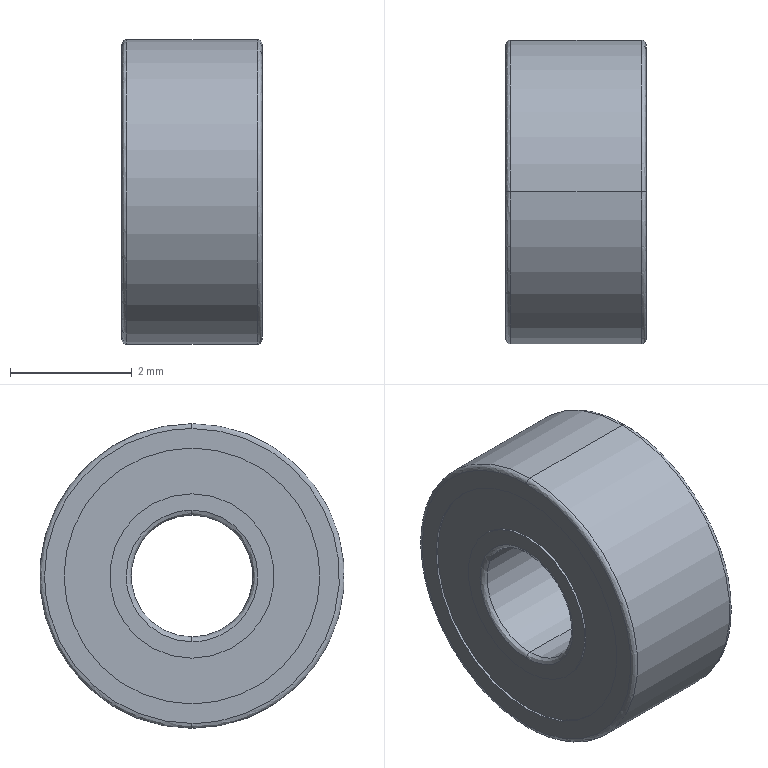Part | SolidWorks | features BaseBody 1 | 1 solid | 26 faces | box 2.3 x 5 x 5 mm | volume 37.258 mm3 | cylinder 12 | spline 8 | plane 6 | commonest cylinder face diameters 2.7 x4 4.2 x4 2 x2 5 x2
STEP:
#1=CARTESIAN_POINT('',(2.22,0.,-2.5));
#2=VERTEX_POINT('',#1);
#3=CARTESIAN_POINT('',(2.22,0.,2.5));
#4=VERTEX_POINT('',#3);
#5=CARTESIAN_POINT('',(2.22,0.,0.));
#6=DIRECTION('',(-1.,0.,0.));
#7=DIRECTION('',(0.,0.,-1.));
#8=AXIS2_PLACEMENT_3D('',#5,#6,#7);
#9=CIRCLE('',#8,2.5);
#10=EDGE_CURVE('',#2,#4,#9,.T.);
#11=ORIENTED_EDGE('',*,*,#10,.F.);
#12=CARTESIAN_POINT('',(2.3,0.,-2.42));
#13=VERTEX_POINT('',#12);
#14=CARTESIAN_POINT('',(2.22,0.,-2.42));
#15=DIRECTION('',(0.,-1.,0.));
#16=DIRECTION('',(0.,0.,-1.));
#17=AXIS2_PLACEMENT_3D('',#14,#15,#16);
#18=CIRCLE('',#17,0.08);
#19=EDGE_CURVE('',#2,#13,#18,.T.);
#20=ORIENTED_EDGE('',*,*,#19,.T.);
#21=CARTESIAN_POINT('',(2.3,0.,2.42));
#22=VERTEX_POINT('',#21);
#23=CARTESIAN_POINT('',(2.3,0.,-2.42));
#24=CARTESIAN_POINT('',(2.3,-4.84,-2.42));
#25=CARTESIAN_POINT('',(2.3,-4.84,2.42));
#26=CARTESIAN_POINT('',(2.3,0.,2.42));
#27=(BOUNDED_CURVE()B_SPLINE_CURVE(3,(#23,#24,#25,#26),.UNSPECIFIED.,.F.,.F.)B_SPLINE_CURVE_WITH_KNOTS((4,4),(0.,1.),.UNSPECIFIED.)CURVE()GEOMETRIC_REPRESENTATION_ITEM()RATIONAL_B_SPLINE_CURVE((1.,0.3333,0.3333,1.))REPRESENTATION_ITEM(''));
#28=EDGE_CURVE('',#13,#22,#27,.T.);
#29=ORIENTED_EDGE('',*,*,#28,.T.);
#30=CARTESIAN_POINT('',(2.22,0.,2.42));
#31=DIRECTION('',(0.,1.,0.));
#32=DIRECTION('',(0.,0.,1.));
#33=AXIS2_PLACEMENT_3D('',#30,#31,#32);
#34=CIRCLE('',#33,0.08);
#35=EDGE_CURVE('',#4,#22,#34,.T.);
#36=ORIENTED_EDGE('',*,*,#35,.F.);
#37=EDGE_LOOP('',(#11,#20,#29,#36));
#38=FACE_OUTER_BOUND('',#37,.T.);
#39=CARTESIAN_POINT('',(2.22,0.,-2.5));
#40=CARTESIAN_POINT('',(2.22,-5.,-2.5));
#41=CARTESIAN_POINT('',(2.22,-5.,2.5));
#42=CARTESIAN_POINT('',(2.22,0.,2.5));
#43=CARTESIAN_POINT('',(2.267,0.,-2.5));
#44=CARTESIAN_POINT('',(2.267,-5.,-2.5));
#45=CARTESIAN_POINT('',(2.267,-5.,2.5));
#46=CARTESIAN_POINT('',(2.267,0.,2.5));
#47=CARTESIAN_POINT('',(2.3,0.,-2.467));
#48=CARTESIAN_POINT('',(2.3,-4.934,-2.467));
#49=CARTESIAN_POINT('',(2.3,-4.934,2.467));
#50=CARTESIAN_POINT('',(2.3,0.,2.467));
#51=CARTESIAN_POINT('',(2.3,0.,-2.42));
#52=CARTESIAN_POINT('',(2.3,-4.84,-2.42));
#53=CARTESIAN_POINT('',(2.3,-4.84,2.42));
#54=CARTESIAN_POINT('',(2.3,0.,2.42));
#55=(BOUNDED_SURFACE()B_SPLINE_SURFACE(3,3,((#39,#40,#41,#42),(#43,#44,#45,#46),(#47,#48,#49,#50),(#51,#52,#53,#54)),.UNSPECIFIED.,.F.,.F.,.T.)B_SPLINE_SURFACE_WITH_KNOTS((4,4),(4,4),(0.,1.),(0.,1.),.UNSPECIFIED.)GEOMETRIC_REPRESENTATION_ITEM()RATIONAL_B_SPLINE_SURFACE(((1.,0.3333,0.3333,1.),(0.8047,0.2682,0.2682,0.8047),(0.8047,0.2682,0.2682,0.8047),(1.,0.3333,0.3333,1.)))REPRESENTATION_ITEM('')SURFACE());
#56=ADVANCED_FACE('',(#38),#55,.T.);
#57=CARTESIAN_POINT('',(0.,0.,2.42));
#58=VERTEX_POINT('',#57);
#59=CARTESIAN_POINT('',(0.,0.,-2.42));
#60=VERTEX_POINT('',#59);
#61=CARTESIAN_POINT('',(0.,0.,2.42));
#62=CARTESIAN_POINT('',(0.,-4.84,2.42));
#63=CARTESIAN_POINT('',(0.,-4.84,-2.42));
#64=CARTESIAN_POINT('',(0.,0.,-2.42));
#65=(BOUNDED_CURVE()B_SPLINE_CURVE(3,(#61,#62,#63,#64),.UNSPECIFIED.,.F.,.T.)B_SPLINE_CURVE_WITH_KNOTS((4,4),(0.,1.),.UNSPECIFIED.)CURVE()GEOMETRIC_REPRESENTATION_ITEM()RATIONAL_B_SPLINE_CURVE((1.,0.3333,0.3333,1.))REPRESENTATION_ITEM(''));
#66=EDGE_CURVE('',#58,#60,#65,.T.);
#67=ORIENTED_EDGE('',*,*,#66,.T.);
#68=CARTESIAN_POINT('',(0.08,0.,-2.5));
#69=VERTEX_POINT('',#68);
#70=CARTESIAN_POINT('',(0.08,0.,-2.42));
#71=DIRECTION('',(0.,-1.,0.));
#72=DIRECTION('',(0.,0.,-1.));
#73=AXIS2_PLACEMENT_3D('',#70,#71,#72);
#74=CIRCLE('',#73,0.08);
#75=EDGE_CURVE('',#60,#69,#74,.T.);
#76=ORIENTED_EDGE('',*,*,#75,.T.);
#77=CARTESIAN_POINT('',(0.08,0.,2.5));
#78=VERTEX_POINT('',#77);
#79=CARTESIAN_POINT('',(0.08,0.,0.));
#80=DIRECTION('',(1.,0.,0.));
#81=DIRECTION('',(0.,0.,-1.));
#82=AXIS2_PLACEMENT_3D('',#79,#80,#81);
#83=CIRCLE('',#82,2.5);
#84=EDGE_CURVE('',#78,#69,#83,.T.);
#85=ORIENTED_EDGE('',*,*,#84,.F.);
#86=CARTESIAN_POINT('',(0.08,0.,2.42));
#87=DIRECTION('',(0.,1.,0.));
#88=DIRECTION('',(0.,0.,1.));
#89=AXIS2_PLACEMENT_3D('',#86,#87,#88);
#90=CIRCLE('',#89,0.08);
#91=EDGE_CURVE('',#58,#78,#90,.T.);
#92=ORIENTED_EDGE('',*,*,#91,.F.);
#93=EDGE_LOOP('',(#67,#76,#85,#92));
#94=FACE_OUTER_BOUND('',#93,.T.);
#95=CARTESIAN_POINT('',(0.,0.,-2.42));
#96=CARTESIAN_POINT('',(0.,-4.84,-2.42));
#97=CARTESIAN_POINT('',(0.,-4.84,2.42));
#98=CARTESIAN_POINT('',(0.,0.,2.42));
#99=CARTESIAN_POINT('',(0.,0.,-2.467));
#100=CARTESIAN_POINT('',(0.,-4.934,-2.467));
#101=CARTESIAN_POINT('',(0.,-4.934,2.467));
#102=CARTESIAN_POINT('',(0.,0.,2.467));
#103=CARTESIAN_POINT('',(0.03314,0.,-2.5));
#104=CARTESIAN_POINT('',(0.03314,-5.,-2.5));
#105=CARTESIAN_POINT('',(0.03314,-5.,2.5));
#106=CARTESIAN_POINT('',(0.03314,0.,2.5));
#107=CARTESIAN_POINT('',(0.08,0.,-2.5));
#108=CARTESIAN_POINT('',(0.08,-5.,-2.5));
#109=CARTESIAN_POINT('',(0.08,-5.,2.5));
#110=CARTESIAN_POINT('',(0.08,0.,2.5));
#111=(BOUNDED_SURFACE()B_SPLINE_SURFACE(3,3,((#95,#96,#97,#98),(#99,#100,#101,#102),(#103,#104,#105,#106),(#107,#108,#109,#110)),.UNSPECIFIED.,.F.,.F.,.F.)B_SPLINE_SURFACE_WITH_KNOTS((4,4),(4,4),(0.,1.),(0.,1.),.UNSPECIFIED.)GEOMETRIC_REPRESENTATION_ITEM()RATIONAL_B_SPLINE_SURFACE(((1.,0.3333,0.3333,1.),(0.8047,0.2682,0.2682,0.8047),(0.8047,0.2682,0.2682,0.8047),(1.,0.3333,0.3333,1.)))REPRESENTATION_ITEM('')SURFACE());
#112=ADVANCED_FACE('',(#94),#111,.T.);
#113=CARTESIAN_POINT('',(2.3,0.,-1.08));
#114=VERTEX_POINT('',#113);
#115=CARTESIAN_POINT('',(2.3,0.,1.08));
#116=VERTEX_POINT('',#115);
#117=CARTESIAN_POINT('',(2.3,0.,-1.08));
#118=CARTESIAN_POINT('',(2.3,-0.06875,-1.08));
#119=CARTESIAN_POINT('',(2.3,-0.17,-1.07));
#120=CARTESIAN_POINT('',(2.3,-0.2849,-1.043));
#121=CARTESIAN_POINT('',(2.3,-0.3334,-1.027));
#122=CARTESIAN_POINT('',(2.3,-0.3656,-1.016));
#123=CARTESIAN_POINT('',(2.3,-0.3802,-1.011));
#124=CARTESIAN_POINT('',(2.3,-0.5359,-0.9495));
#125=CARTESIAN_POINT('',(2.3,-0.6584,-0.8688));
#126=CARTESIAN_POINT('',(2.3,-0.8163,-0.7111));
#127=CARTESIAN_POINT('',(2.3,-0.8858,-0.6259));
#128=CARTESIAN_POINT('',(2.3,-0.9505,-0.5154));
#129=CARTESIAN_POINT('',(2.3,-0.9747,-0.4657));
#130=CARTESIAN_POINT('',(2.3,-0.99,-0.432));
#131=CARTESIAN_POINT('',(2.3,-0.9979,-0.4135));
#132=CARTESIAN_POINT('',(2.3,-1.055,-0.2702));
#133=CARTESIAN_POINT('',(2.3,-1.08,-0.137));
#134=CARTESIAN_POINT('',(2.3,-1.08,0.06849));
#135=CARTESIAN_POINT('',(2.3,-1.071,0.1696));
#136=CARTESIAN_POINT('',(2.3,-1.043,0.2845));
#137=CARTESIAN_POINT('',(2.3,-1.028,0.3332));
#138=CARTESIAN_POINT('',(2.3,-1.016,0.3655));
#139=CARTESIAN_POINT('',(2.3,-1.011,0.3802));
#140=CARTESIAN_POINT('',(2.3,-0.9495,0.5359));
#141=CARTESIAN_POINT('',(2.3,-0.8688,0.6584));
#142=CARTESIAN_POINT('',(2.3,-0.7111,0.8163));
#143=CARTESIAN_POINT('',(2.3,-0.6259,0.8858));
#144=CARTESIAN_POINT('',(2.3,-0.5154,0.9505));
#145=CARTESIAN_POINT('',(2.3,-0.4657,0.9747));
#146=CARTESIAN_POINT('',(2.3,-0.432,0.99));
#147=CARTESIAN_POINT('',(2.3,-0.4134,0.9979));
#148=CARTESIAN_POINT('',(2.3,-0.2704,1.055));
#149=CARTESIAN_POINT('',(2.3,-0.1379,1.08));
#150=CARTESIAN_POINT('',(2.3,0.,1.08));
#151=B_SPLINE_CURVE_WITH_KNOTS('',3,(#117,#118,#119,#120,#121,#122,#123,#124,#125,#126,#127,#128,#129,#130,#131,#132,#133,#134,#135,#136,#137,#138,#139,#140,#141,#142,#143,#144,#145,#146,#147,#148,#149,#150),.UNSPECIFIED.,.F.,.F.,(4,1,1,2,2,2,1,1,2,2,2,1,1,2,2,2,1,1,2,2,4),(0.,0.0625,0.09375,0.1094,0.125,0.25,0.3125,0.3438,0.3594,0.375,0.5,0.5625,0.5938,0.6094,0.625,0.75,0.8125,0.8438,0.8594,0.875,1.),.UNSPECIFIED.);
#152=EDGE_CURVE('',#114,#116,#151,.T.);
#153=ORIENTED_EDGE('',*,*,#152,.F.);
#154=CARTESIAN_POINT('',(2.22,0.,-1.));
#155=VERTEX_POINT('',#154);
#156=CARTESIAN_POINT('',(2.22,0.,-1.08));
#157=DIRECTION('',(0.,-1.,0.));
#158=DIRECTION('',(0.,0.,-1.));
#159=AXIS2_PLACEMENT_3D('',#156,#157,#158);
#160=CIRCLE('',#159,0.08);
#161=EDGE_CURVE('',#114,#155,#160,.T.);
#162=ORIENTED_EDGE('',*,*,#161,.T.);
#163=CARTESIAN_POINT('',(2.22,0.,1.));
#164=VERTEX_POINT('',#163);
#165=CARTESIAN_POINT('',(2.22,0.,0.));
#166=DIRECTION('',(-1.,0.,0.));
#167=DIRECTION('',(0.,0.,1.));
#168=AXIS2_PLACEMENT_3D('',#165,#166,#167);
#169=CIRCLE('',#168,1.);
#170=EDGE_CURVE('',#155,#164,#169,.T.);
#171=ORIENTED_EDGE('',*,*,#170,.T.);
#172=CARTESIAN_POINT('',(2.22,0.,1.08));
#173=DIRECTION('',(0.,1.,0.));
#174=DIRECTION('',(0.,0.,1.));
#175=AXIS2_PLACEMENT_3D('',#172,#173,#174);
#176=CIRCLE('',#175,0.08);
#177=EDGE_CURVE('',#116,#164,#176,.T.);
#178=ORIENTED_EDGE('',*,*,#177,.F.);
#179=EDGE_LOOP('',(#153,#162,#171,#178));
#180=FACE_OUTER_BOUND('',#179,.T.);
#181=CARTESIAN_POINT('',(2.3,0.,-1.08));
#182=CARTESIAN_POINT('',(2.3,-2.16,-1.08));
#183=CARTESIAN_POINT('',(2.3,-2.16,1.08));
#184=CARTESIAN_POINT('',(2.3,0.,1.08));
#185=CARTESIAN_POINT('',(2.3,0.,-1.033));
#186=CARTESIAN_POINT('',(2.3,-2.066,-1.033));
#187=CARTESIAN_POINT('',(2.3,-2.066,1.033));
#188=CARTESIAN_POINT('',(2.3,0.,1.033));
#189=CARTESIAN_POINT('',(2.267,0.,-1.));
#190=CARTESIAN_POINT('',(2.267,-2.,-1.));
#191=CARTESIAN_POINT('',(2.267,-2.,1.));
#192=CARTESIAN_POINT('',(2.267,0.,1.));
#193=CARTESIAN_POINT('',(2.22,0.,-1.));
#194=CARTESIAN_POINT('',(2.22,-2.,-1.));
#195=CARTESIAN_POINT('',(2.22,-2.,1.));
#196=CARTESIAN_POINT('',(2.22,0.,1.));
#197=(BOUNDED_SURFACE()B_SPLINE_SURFACE(3,3,((#181,#182,#183,#184),(#185,#186,#187,#188),(#189,#190,#191,#192),(#193,#194,#195,#196)),.UNSPECIFIED.,.F.,.F.,.T.)B_SPLINE_SURFACE_WITH_KNOTS((4,4),(4,4),(0.,1.),(0.,1.),.UNSPECIFIED.)GEOMETRIC_REPRESENTATION_ITEM()RATIONAL_B_SPLINE_SURFACE(((1.,0.3333,0.3333,1.),(0.8047,0.2682,0.2682,0.8047),(0.8047,0.2682,0.2682,0.8047),(1.,0.3333,0.3333,1.)))REPRESENTATION_ITEM('')SURFACE());
#198=ADVANCED_FACE('',(#180),#197,.T.);
#199=CARTESIAN_POINT('',(0.08,0.,1.));
#200=VERTEX_POINT('',#199);
#201=CARTESIAN_POINT('',(0.08,0.,-1.));
#202=VERTEX_POINT('',#201);
#203=CARTESIAN_POINT('',(0.08,0.,0.));
#204=DIRECTION('',(1.,0.,0.));
#205=DIRECTION('',(0.,0.,1.));
#206=AXIS2_PLACEMENT_3D('',#203,#204,#205);
#207=CIRCLE('',#206,1.);
#208=EDGE_CURVE('',#200,#202,#207,.T.);
#209=ORIENTED_EDGE('',*,*,#208,.T.);
#210=CARTESIAN_POINT('',(0.,0.,-1.08));
#211=VERTEX_POINT('',#210);
#212=CARTESIAN_POINT('',(0.08,0.,-1.08));
#213=DIRECTION('',(0.,-1.,0.));
#214=DIRECTION('',(0.,0.,-1.));
#215=AXIS2_PLACEMENT_3D('',#212,#213,#214);
#216=CIRCLE('',#215,0.08);
#217=EDGE_CURVE('',#202,#211,#216,.T.);
#218=ORIENTED_EDGE('',*,*,#217,.T.);
#219=CARTESIAN_POINT('',(0.,0.,1.08));
#220=VERTEX_POINT('',#219);
#221=CARTESIAN_POINT('',(0.,0.,1.08));
#222=CARTESIAN_POINT('',(0.,-0.06875,1.08));
#223=CARTESIAN_POINT('',(0.,-0.17,1.07));
#224=CARTESIAN_POINT('',(0.,-0.2849,1.043));
#225=CARTESIAN_POINT('',(0.,-0.3334,1.027));
#226=CARTESIAN_POINT('',(0.,-0.3656,1.016));
#227=CARTESIAN_POINT('',(0.,-0.3802,1.011));
#228=CARTESIAN_POINT('',(0.,-0.5359,0.9495));
#229=CARTESIAN_POINT('',(0.,-0.6584,0.8688));
#230=CARTESIAN_POINT('',(0.,-0.8163,0.7111));
#231=CARTESIAN_POINT('',(0.,-0.8858,0.6259));
#232=CARTESIAN_POINT('',(0.,-0.9505,0.5154));
#233=CARTESIAN_POINT('',(0.,-0.9747,0.4657));
#234=CARTESIAN_POINT('',(0.,-0.99,0.432));
#235=CARTESIAN_POINT('',(0.,-0.9979,0.4135));
#236=CARTESIAN_POINT('',(0.,-1.055,0.2702));
#237=CARTESIAN_POINT('',(0.,-1.08,0.137));
#238=CARTESIAN_POINT('',(0.,-1.08,-0.06849));
#239=CARTESIAN_POINT('',(0.,-1.071,-0.1696));
#240=CARTESIAN_POINT('',(0.,-1.043,-0.2845));
#241=CARTESIAN_POINT('',(0.,-1.028,-0.3332));
#242=CARTESIAN_POINT('',(0.,-1.016,-0.3655));
#243=CARTESIAN_POINT('',(0.,-1.011,-0.3802));
#244=CARTESIAN_POINT('',(0.,-0.9495,-0.5359));
#245=CARTESIAN_POINT('',(0.,-0.8688,-0.6584));
#246=CARTESIAN_POINT('',(0.,-0.7111,-0.8163));
#247=CARTESIAN_POINT('',(0.,-0.6259,-0.8858));
#248=CARTESIAN_POINT('',(0.,-0.5154,-0.9505));
#249=CARTESIAN_POINT('',(0.,-0.4657,-0.9747));
#250=CARTESIAN_POINT('',(0.,-0.432,-0.99));
#251=CARTESIAN_POINT('',(0.,-0.4134,-0.9979));
#252=CARTESIAN_POINT('',(0.,-0.2704,-1.055));
#253=CARTESIAN_POINT('',(0.,-0.1379,-1.08));
#254=CARTESIAN_POINT('',(0.,0.,-1.08));
#255=B_SPLINE_CURVE_WITH_KNOTS('',3,(#221,#222,#223,#224,#225,#226,#227,#228,#229,#230,#231,#232,#233,#234,#235,#236,#237,#238,#239,#240,#241,#242,#243,#244,#245,#246,#247,#248,#249,#250,#251,#252,#253,#254),.UNSPECIFIED.,.F.,.F.,(4,1,1,2,2,2,1,1,2,2,2,1,1,2,2,2,1,1,2,2,4),(0.,0.0625,0.09375,0.1094,0.125,0.25,0.3125,0.3438,0.3594,0.375,0.5,0.5625,0.5938,0.6094,0.625,0.75,0.8125,0.8438,0.8594,0.875,1.),.UNSPECIFIED.);
#256=EDGE_CURVE('',#220,#211,#255,.T.);
#257=ORIENTED_EDGE('',*,*,#256,.F.);
#258=CARTESIAN_POINT('',(0.08,0.,1.08));
#259=DIRECTION('',(0.,1.,0.));
#260=DIRECTION('',(0.,0.,1.));
#261=AXIS2_PLACEMENT_3D('',#258,#259,#260);
#262=CIRCLE('',#261,0.08);
#263=EDGE_CURVE('',#200,#220,#262,.T.);
#264=ORIENTED_EDGE('',*,*,#263,.F.);
#265=EDGE_LOOP('',(#209,#218,#257,#264));
#266=FACE_OUTER_BOUND('',#265,.T.);
#267=CARTESIAN_POINT('',(0.08,0.,-1.));
#268=CARTESIAN_POINT('',(0.08,-2.,-1.));
#269=CARTESIAN_POINT('',(0.08,-2.,1.));
#270=CARTESIAN_POINT('',(0.08,0.,1.));
#271=CARTESIAN_POINT('',(0.03314,0.,-1.));
#272=CARTESIAN_POINT('',(0.03314,-2.,-1.));
#273=CARTESIAN_POINT('',(0.03314,-2.,1.));
#274=CARTESIAN_POINT('',(0.03314,0.,1.));
#275=CARTESIAN_POINT('',(0.,0.,-1.033));
#276=CARTESIAN_POINT('',(0.,-2.066,-1.033));
#277=CARTESIAN_POINT('',(0.,-2.066,1.033));
#278=CARTESIAN_POINT('',(0.,0.,1.033));
#279=CARTESIAN_POINT('',(0.,0.,-1.08));
#280=CARTESIAN_POINT('',(0.,-2.16,-1.08));
#281=CARTESIAN_POINT('',(0.,-2.16,1.08));
#282=CARTESIAN_POINT('',(0.,0.,1.08));
#283=(BOUNDED_SURFACE()B_SPLINE_SURFACE(3,3,((#267,#268,#269,#270),(#271,#272,#273,#274),(#275,#276,#277,#278),(#279,#280,#281,#282)),.UNSPECIFIED.,.F.,.F.,.F.)B_SPLINE_SURFACE_WITH_KNOTS((4,4),(4,4),(0.,1.),(0.,1.),.UNSPECIFIED.)GEOMETRIC_REPRESENTATION_ITEM()RATIONAL_B_SPLINE_SURFACE(((1.,0.3333,0.3333,1.),(0.8047,0.2682,0.2682,0.8047),(0.8047,0.2682,0.2682,0.8047),(1.,0.3333,0.3333,1.)))REPRESENTATION_ITEM('')SURFACE());
#284=ADVANCED_FACE('',(#266),#283,.T.);
#285=CARTESIAN_POINT('',(0.08,0.,0.));
#286=DIRECTION('',(1.,0.,0.));
#287=DIRECTION('',(0.,0.,-1.));
#288=AXIS2_PLACEMENT_3D('',#285,#286,#287);
#289=CIRCLE('',#288,2.5);
#290=EDGE_CURVE('',#69,#78,#289,.T.);
#291=ORIENTED_EDGE('',*,*,#290,.T.);
#292=CARTESIAN_POINT('',(1.15,0.,2.5));
#293=DIRECTION('',(1.,0.,0.));
#294=VECTOR('',#293,1000.);
#295=LINE('',#292,#294);
#296=EDGE_CURVE('',#78,#4,#295,.T.);
#297=ORIENTED_EDGE('',*,*,#296,.T.);
#298=CARTESIAN_POINT('',(2.22,0.,0.));
#299=DIRECTION('',(-1.,0.,0.));
#300=DIRECTION('',(0.,0.,-1.));
#301=AXIS2_PLACEMENT_3D('',#298,#299,#300);
#302=CIRCLE('',#301,2.5);
#303=EDGE_CURVE('',#4,#2,#302,.T.);
#304=ORIENTED_EDGE('',*,*,#303,.T.);
#305=CARTESIAN_POINT('',(1.15,0.,-2.5));
#306=DIRECTION('',(1.,0.,0.));
#307=VECTOR('',#306,1000.);
#308=LINE('',#305,#307);
#309=EDGE_CURVE('',#69,#2,#308,.T.);
#310=ORIENTED_EDGE('',*,*,#309,.F.);
#311=EDGE_LOOP('',(#291,#297,#304,#310));
#312=FACE_OUTER_BOUND('',#311,.T.);
#313=CARTESIAN_POINT('',(1.15,0.,0.));
#314=DIRECTION('',(1.,0.,0.));
#315=DIRECTION('',(0.,0.,-1.));
#316=AXIS2_PLACEMENT_3D('',#313,#314,#315);
#317=CYLINDRICAL_SURFACE('',#316,2.5);
#318=ADVANCED_FACE('',(#312),#317,.T.);
#319=CARTESIAN_POINT('',(2.262,0.,2.1));
#320=VERTEX_POINT('',#319);
#321=CARTESIAN_POINT('',(2.262,0.,-2.1));
#322=VERTEX_POINT('',#321);
#323=CARTESIAN_POINT('',(2.262,0.,0.));
#324=DIRECTION('',(1.,0.,0.));
#325=DIRECTION('',(0.,0.,-1.));
#326=AXIS2_PLACEMENT_3D('',#323,#324,#325);
#327=CIRCLE('',#326,2.1);
#328=EDGE_CURVE('',#320,#322,#327,.T.);
#329=ORIENTED_EDGE('',*,*,#328,.F.);
#330=CARTESIAN_POINT('',(2.3,0.,2.1));
#331=VERTEX_POINT('',#330);
#332=CARTESIAN_POINT('',(2.281,0.,2.1));
#333=DIRECTION('',(1.,0.,0.));
#334=VECTOR('',#333,1000.);
#335=LINE('',#332,#334);
#336=EDGE_CURVE('',#320,#331,#335,.T.);
#337=ORIENTED_EDGE('',*,*,#336,.T.);
#338=CARTESIAN_POINT('',(2.3,0.,-2.1));
#339=VERTEX_POINT('',#338);
#340=CARTESIAN_POINT('',(2.3,0.,0.));
#341=DIRECTION('',(-1.,0.,0.));
#342=DIRECTION('',(0.,0.,-1.));
#343=AXIS2_PLACEMENT_3D('',#340,#341,#342);
#344=CIRCLE('',#343,2.1);
#345=EDGE_CURVE('',#339,#331,#344,.T.);
#346=ORIENTED_EDGE('',*,*,#345,.F.);
#347=CARTESIAN_POINT('',(2.281,0.,-2.1));
#348=DIRECTION('',(1.,0.,0.));
#349=VECTOR('',#348,1000.);
#350=LINE('',#347,#349);
#351=EDGE_CURVE('',#322,#339,#350,.T.);
#352=ORIENTED_EDGE('',*,*,#351,.F.);
#353=EDGE_LOOP('',(#329,#337,#346,#352));
#354=FACE_OUTER_BOUND('',#353,.T.);
#355=CARTESIAN_POINT('',(2.281,0.,0.));
#356=DIRECTION('',(1.,0.,0.));
#357=DIRECTION('',(0.,0.,-1.));
#358=AXIS2_PLACEMENT_3D('',#355,#356,#357);
#359=CYLINDRICAL_SURFACE('',#358,2.1);
#360=ADVANCED_FACE('',(#354),#359,.F.);
#361=CARTESIAN_POINT('',(0.,0.,2.1));
#362=VERTEX_POINT('',#361);
#363=CARTESIAN_POINT('',(0.,0.,-2.1));
#364=VERTEX_POINT('',#363);
#365=CARTESIAN_POINT('',(0.,0.,0.));
#366=DIRECTION('',(1.,0.,0.));
#367=DIRECTION('',(0.,0.,-1.));
#368=AXIS2_PLACEMENT_3D('',#365,#366,#367);
#369=CIRCLE('',#368,2.1);
#370=EDGE_CURVE('',#362,#364,#369,.T.);
#371=ORIENTED_EDGE('',*,*,#370,.F.);
#372=CARTESIAN_POINT('',(0.0382,0.,2.1));
#373=VERTEX_POINT('',#372);
#374=CARTESIAN_POINT('',(0.0191,0.,2.1));
#375=DIRECTION('',(1.,0.,0.));
#376=VECTOR('',#375,1000.);
#377=LINE('',#374,#376);
#378=EDGE_CURVE('',#362,#373,#377,.T.);
#379=ORIENTED_EDGE('',*,*,#378,.T.);
#380=CARTESIAN_POINT('',(0.0382,0.,-2.1));
#381=VERTEX_POINT('',#380);
#382=CARTESIAN_POINT('',(0.0382,0.,0.));
#383=DIRECTION('',(-1.,0.,0.));
#384=DIRECTION('',(0.,0.,-1.));
#385=AXIS2_PLACEMENT_3D('',#382,#383,#384);
#386=CIRCLE('',#385,2.1);
#387=EDGE_CURVE('',#381,#373,#386,.T.);
#388=ORIENTED_EDGE('',*,*,#387,.F.);
#389=CARTESIAN_POINT('',(0.0191,0.,-2.1));
#390=DIRECTION('',(1.,0.,0.));
#391=VECTOR('',#390,1000.);
#392=LINE('',#389,#391);
#393=EDGE_CURVE('',#364,#381,#392,.T.);
#394=ORIENTED_EDGE('',*,*,#393,.F.);
#395=EDGE_LOOP('',(#371,#379,#388,#394));
#396=FACE_OUTER_BOUND('',#395,.T.);
#397=CARTESIAN_POINT('',(0.0191,0.,0.));
#398=DIRECTION('',(1.,0.,0.));
#399=DIRECTION('',(0.,0.,-1.));
#400=AXIS2_PLACEMENT_3D('',#397,#398,#399);
#401=CYLINDRICAL_SURFACE('',#400,2.1);
#402=ADVANCED_FACE('',(#396),#401,.F.);
#403=CARTESIAN_POINT('',(2.262,0.,1.35));
#404=VERTEX_POINT('',#403);
#405=CARTESIAN_POINT('',(2.262,0.,-1.35));
#406=VERTEX_POINT('',#405);
#407=CARTESIAN_POINT('',(2.262,0.,0.));
#408=DIRECTION('',(-1.,0.,0.));
#409=DIRECTION('',(0.,0.,-1.));
#410=AXIS2_PLACEMENT_3D('',#407,#408,#409);
#411=CIRCLE('',#410,1.35);
#412=EDGE_CURVE('',#404,#406,#411,.T.);
#413=ORIENTED_EDGE('',*,*,#412,.F.);
#414=CARTESIAN_POINT('',(2.3,0.,1.35));
#415=VERTEX_POINT('',#414);
#416=CARTESIAN_POINT('',(2.281,0.,1.35));
#417=DIRECTION('',(1.,0.,0.));
#418=VECTOR('',#417,1000.);
#419=LINE('',#416,#418);
#420=EDGE_CURVE('',#404,#415,#419,.T.);
#421=ORIENTED_EDGE('',*,*,#420,.T.);
#422=CARTESIAN_POINT('',(2.3,0.,-1.35));
#423=VERTEX_POINT('',#422);
#424=CARTESIAN_POINT('',(2.3,0.,0.));
#425=DIRECTION('',(-1.,0.,0.));
#426=DIRECTION('',(0.,0.,-1.));
#427=AXIS2_PLACEMENT_3D('',#424,#425,#426);
#428=CIRCLE('',#427,1.35);
#429=EDGE_CURVE('',#415,#423,#428,.T.);
#430=ORIENTED_EDGE('',*,*,#429,.T.);
#431=CARTESIAN_POINT('',(2.281,0.,-1.35));
#432=DIRECTION('',(1.,0.,0.));
#433=VECTOR('',#432,1000.);
#434=LINE('',#431,#433);
#435=EDGE_CURVE('',#406,#423,#434,.T.);
#436=ORIENTED_EDGE('',*,*,#435,.F.);
#437=EDGE_LOOP('',(#413,#421,#430,#436));
#438=FACE_OUTER_BOUND('',#437,.T.);
#439=CARTESIAN_POINT('',(2.281,0.,0.));
#440=DIRECTION('',(1.,0.,0.));
#441=DIRECTION('',(0.,0.,-1.));
#442=AXIS2_PLACEMENT_3D('',#439,#440,#441);
#443=CYLINDRICAL_SURFACE('',#442,1.35);
#444=ADVANCED_FACE('',(#438),#443,.T.);
#445=CARTESIAN_POINT('',(0.,0.,-1.35));
#446=VERTEX_POINT('',#445);
#447=CARTESIAN_POINT('',(0.,0.,1.35));
#448=VERTEX_POINT('',#447);
#449=CARTESIAN_POINT('',(0.,0.,0.));
#450=DIRECTION('',(1.,0.,0.));
#451=DIRECTION('',(0.,0.,-1.));
#452=AXIS2_PLACEMENT_3D('',#449,#450,#451);
#453=CIRCLE('',#452,1.35);
#454=EDGE_CURVE('',#446,#448,#453,.T.);
#455=ORIENTED_EDGE('',*,*,#454,.T.);
#456=CARTESIAN_POINT('',(0.0382,0.,1.35));
#457=VERTEX_POINT('',#456);
#458=CARTESIAN_POINT('',(0.0191,0.,1.35));
#459=DIRECTION('',(1.,0.,0.));
#460=VECTOR('',#459,1000.);
#461=LINE('',#458,#460);
#462=EDGE_CURVE('',#448,#457,#461,.T.);
#463=ORIENTED_EDGE('',*,*,#462,.T.);
#464=CARTESIAN_POINT('',(0.0382,0.,-1.35));
#465=VERTEX_POINT('',#464);
#466=CARTESIAN_POINT('',(0.0382,0.,0.));
#467=DIRECTION('',(1.,0.,0.));
#468=DIRECTION('',(0.,0.,-1.));
#469=AXIS2_PLACEMENT_3D('',#466,#467,#468);
#470=CIRCLE('',#469,1.35);
#471=EDGE_CURVE('',#465,#457,#470,.T.);
#472=ORIENTED_EDGE('',*,*,#471,.F.);
#473=CARTESIAN_POINT('',(0.0191,0.,-1.35));
#474=DIRECTION('',(1.,0.,0.));
#475=VECTOR('',#474,1000.);
#476=LINE('',#473,#475);
#477=EDGE_CURVE('',#446,#465,#476,.T.);
#478=ORIENTED_EDGE('',*,*,#477,.F.);
#479=EDGE_LOOP('',(#455,#463,#472,#478));
#480=FACE_OUTER_BOUND('',#479,.T.);
#481=CARTESIAN_POINT('',(0.0191,0.,0.));
#482=DIRECTION('',(1.,0.,0.));
#483=DIRECTION('',(0.,0.,-1.));
#484=AXIS2_PLACEMENT_3D('',#481,#482,#483);
#485=CYLINDRICAL_SURFACE('',#484,1.35);
#486=ADVANCED_FACE('',(#480),#485,.T.);
#487=ORIENTED_EDGE('',*,*,#208,.F.);
#488=CARTESIAN_POINT('',(1.15,0.,1.));
#489=DIRECTION('',(1.,0.,0.));
#490=VECTOR('',#489,1000.);
#491=LINE('',#488,#490);
#492=EDGE_CURVE('',#200,#164,#491,.T.);
#493=ORIENTED_EDGE('',*,*,#492,.T.);
#494=ORIENTED_EDGE('',*,*,#170,.F.);
#495=CARTESIAN_POINT('',(1.15,0.,-1.));
#496=DIRECTION('',(1.,0.,0.));
#497=VECTOR('',#496,1000.);
#498=LINE('',#495,#497);
#499=EDGE_CURVE('',#202,#155,#498,.T.);
#500=ORIENTED_EDGE('',*,*,#499,.F.);
#501=EDGE_LOOP('',(#487,#493,#494,#500));
#502=FACE_OUTER_BOUND('',#501,.T.);
#503=CARTESIAN_POINT('',(1.15,0.,0.));
#504=DIRECTION('',(1.,0.,0.));
#505=DIRECTION('',(0.,0.,-1.));
#506=AXIS2_PLACEMENT_3D('',#503,#504,#505);
#507=CYLINDRICAL_SURFACE('',#506,1.);
#508=ADVANCED_FACE('',(#502),#507,.F.);
#509=ORIENTED_EDGE('',*,*,#296,.F.);
#510=ORIENTED_EDGE('',*,*,#84,.T.);
#511=ORIENTED_EDGE('',*,*,#309,.T.);
#512=ORIENTED_EDGE('',*,*,#10,.T.);
#513=EDGE_LOOP('',(#509,#510,#511,#512));
#514=FACE_OUTER_BOUND('',#513,.T.);
#515=CARTESIAN_POINT('',(1.15,0.,0.));
#516=DIRECTION('',(1.,0.,0.));
#517=DIRECTION('',(0.,0.,-1.));
#518=AXIS2_PLACEMENT_3D('',#515,#516,#517);
#519=CYLINDRICAL_SURFACE('',#518,2.5);
#520=ADVANCED_FACE('',(#514),#519,.T.);
#521=ORIENTED_EDGE('',*,*,#19,.F.);
#522=ORIENTED_EDGE('',*,*,#303,.F.);
#523=ORIENTED_EDGE('',*,*,#35,.T.);
#524=CARTESIAN_POINT('',(2.3,2.42,0.));
#525=VERTEX_POINT('',#524);
#526=CARTESIAN_POINT('',(2.3,0.,2.42));
#527=CARTESIAN_POINT('',(2.3,1.418,2.42));
#528=CARTESIAN_POINT('',(2.3,2.42,1.418));
#529=CARTESIAN_POINT('',(2.3,2.42,0.));
#530=(BOUNDED_CURVE()B_SPLINE_CURVE(3,(#526,#527,#528,#529),.UNSPECIFIED.,.F.,.T.)B_SPLINE_CURVE_WITH_KNOTS((4,4),(0.,1.),.UNSPECIFIED.)CURVE()GEOMETRIC_REPRESENTATION_ITEM()RATIONAL_B_SPLINE_CURVE((1.,0.8047,0.8047,1.))REPRESENTATION_ITEM(''));
#531=EDGE_CURVE('',#22,#525,#530,.T.);
#532=ORIENTED_EDGE('',*,*,#531,.T.);
#533=CARTESIAN_POINT('',(2.3,2.42,0.));
#534=CARTESIAN_POINT('',(2.3,2.42,-1.418));
#535=CARTESIAN_POINT('',(2.3,1.418,-2.42));
#536=CARTESIAN_POINT('',(2.3,0.,-2.42));
#537=(BOUNDED_CURVE()B_SPLINE_CURVE(3,(#533,#534,#535,#536),.UNSPECIFIED.,.F.,.F.)B_SPLINE_CURVE_WITH_KNOTS((4,4),(0.,1.),.UNSPECIFIED.)CURVE()GEOMETRIC_REPRESENTATION_ITEM()RATIONAL_B_SPLINE_CURVE((1.,0.8047,0.8047,1.))REPRESENTATION_ITEM(''));
#538=EDGE_CURVE('',#525,#13,#537,.T.);
#539=ORIENTED_EDGE('',*,*,#538,.T.);
#540=EDGE_LOOP('',(#521,#522,#523,#532,#539));
#541=FACE_OUTER_BOUND('',#540,.T.);
#542=CARTESIAN_POINT('',(2.22,0.,2.5));
#543=CARTESIAN_POINT('',(2.22,5.,2.5));
#544=CARTESIAN_POINT('',(2.22,5.,-2.5));
#545=CARTESIAN_POINT('',(2.22,0.,-2.5));
#546=CARTESIAN_POINT('',(2.267,0.,2.5));
#547=CARTESIAN_POINT('',(2.267,5.,2.5));
#548=CARTESIAN_POINT('',(2.267,5.,-2.5));
#549=CARTESIAN_POINT('',(2.267,0.,-2.5));
#550=CARTESIAN_POINT('',(2.3,0.,2.467));
#551=CARTESIAN_POINT('',(2.3,4.934,2.467));
#552=CARTESIAN_POINT('',(2.3,4.934,-2.467));
#553=CARTESIAN_POINT('',(2.3,0.,-2.467));
#554=CARTESIAN_POINT('',(2.3,0.,2.42));
#555=CARTESIAN_POINT('',(2.3,4.84,2.42));
#556=CARTESIAN_POINT('',(2.3,4.84,-2.42));
#557=CARTESIAN_POINT('',(2.3,0.,-2.42));
#558=(BOUNDED_SURFACE()B_SPLINE_SURFACE(3,3,((#542,#543,#544,#545),(#546,#547,#548,#549),(#550,#551,#552,#553),(#554,#555,#556,#557)),.UNSPECIFIED.,.F.,.F.,.T.)B_SPLINE_SURFACE_WITH_KNOTS((4,4),(4,4),(0.,1.),(0.,1.),.UNSPECIFIED.)GEOMETRIC_REPRESENTATION_ITEM()RATIONAL_B_SPLINE_SURFACE(((1.,0.3333,0.3333,1.),(0.8047,0.2682,0.2682,0.8047),(0.8047,0.2682,0.2682,0.8047),(1.,0.3333,0.3333,1.)))REPRESENTATION_ITEM('')SURFACE());
#559=ADVANCED_FACE('',(#541),#558,.T.);
#560=ORIENTED_EDGE('',*,*,#75,.F.);
#561=CARTESIAN_POINT('',(0.,2.42,0.));
#562=VERTEX_POINT('',#561);
#563=CARTESIAN_POINT('',(0.,0.,-2.42));
#564=CARTESIAN_POINT('',(0.,1.418,-2.42));
#565=CARTESIAN_POINT('',(0.,2.42,-1.418));
#566=CARTESIAN_POINT('',(0.,2.42,0.));
#567=(BOUNDED_CURVE()B_SPLINE_CURVE(3,(#563,#564,#565,#566),.UNSPECIFIED.,.F.,.T.)B_SPLINE_CURVE_WITH_KNOTS((4,4),(0.,1.),.UNSPECIFIED.)CURVE()GEOMETRIC_REPRESENTATION_ITEM()RATIONAL_B_SPLINE_CURVE((1.,0.8047,0.8047,1.))REPRESENTATION_ITEM(''));
#568=EDGE_CURVE('',#60,#562,#567,.T.);
#569=ORIENTED_EDGE('',*,*,#568,.T.);
#570=CARTESIAN_POINT('',(0.,2.42,0.));
#571=CARTESIAN_POINT('',(0.,2.42,1.418));
#572=CARTESIAN_POINT('',(0.,1.418,2.42));
#573=CARTESIAN_POINT('',(0.,0.,2.42));
#574=(BOUNDED_CURVE()B_SPLINE_CURVE(3,(#570,#571,#572,#573),.UNSPECIFIED.,.F.,.T.)B_SPLINE_CURVE_WITH_KNOTS((4,4),(0.,1.),.UNSPECIFIED.)CURVE()GEOMETRIC_REPRESENTATION_ITEM()RATIONAL_B_SPLINE_CURVE((1.,0.8047,0.8047,1.))REPRESENTATION_ITEM(''));
#575=EDGE_CURVE('',#562,#58,#574,.T.);
#576=ORIENTED_EDGE('',*,*,#575,.T.);
#577=ORIENTED_EDGE('',*,*,#91,.T.);
#578=ORIENTED_EDGE('',*,*,#290,.F.);
#579=EDGE_LOOP('',(#560,#569,#576,#577,#578));
#580=FACE_OUTER_BOUND('',#579,.T.);
#581=CARTESIAN_POINT('',(0.,0.,2.42));
#582=CARTESIAN_POINT('',(0.,4.84,2.42));
#583=CARTESIAN_POINT('',(0.,4.84,-2.42));
#584=CARTESIAN_POINT('',(0.,0.,-2.42));
#585=CARTESIAN_POINT('',(0.,0.,2.467));
#586=CARTESIAN_POINT('',(0.,4.934,2.467));
#587=CARTESIAN_POINT('',(0.,4.934,-2.467));
#588=CARTESIAN_POINT('',(0.,0.,-2.467));
#589=CARTESIAN_POINT('',(0.03314,0.,2.5));
#590=CARTESIAN_POINT('',(0.03314,5.,2.5));
#591=CARTESIAN_POINT('',(0.03314,5.,-2.5));
#592=CARTESIAN_POINT('',(0.03314,0.,-2.5));
#593=CARTESIAN_POINT('',(0.08,0.,2.5));
#594=CARTESIAN_POINT('',(0.08,5.,2.5));
#595=CARTESIAN_POINT('',(0.08,5.,-2.5));
#596=CARTESIAN_POINT('',(0.08,0.,-2.5));
#597=(BOUNDED_SURFACE()B_SPLINE_SURFACE(3,3,((#581,#582,#583,#584),(#585,#586,#587,#588),(#589,#590,#591,#592),(#593,#594,#595,#596)),.UNSPECIFIED.,.F.,.F.,.T.)B_SPLINE_SURFACE_WITH_KNOTS((4,4),(4,4),(0.,1.),(0.,1.),.UNSPECIFIED.)GEOMETRIC_REPRESENTATION_ITEM()RATIONAL_B_SPLINE_SURFACE(((1.,0.3333,0.3333,1.),(0.8047,0.2682,0.2682,0.8047),(0.8047,0.2682,0.2682,0.8047),(1.,0.3333,0.3333,1.)))REPRESENTATION_ITEM('')SURFACE());
#598=ADVANCED_FACE('',(#580),#597,.T.);
#599=ORIENTED_EDGE('',*,*,#345,.T.);
#600=CARTESIAN_POINT('',(2.3,0.,0.));
#601=DIRECTION('',(-1.,0.,0.));
#602=DIRECTION('',(0.,0.,-1.));
#603=AXIS2_PLACEMENT_3D('',#600,#601,#602);
#604=CIRCLE('',#603,2.1);
#605=EDGE_CURVE('',#331,#339,#604,.T.);
#606=ORIENTED_EDGE('',*,*,#605,.T.);
#607=EDGE_LOOP('',(#599,#606));
#608=FACE_BOUND('',#607,.T.);
#609=ORIENTED_EDGE('',*,*,#531,.F.);
#610=ORIENTED_EDGE('',*,*,#28,.F.);
#611=ORIENTED_EDGE('',*,*,#538,.F.);
#612=EDGE_LOOP('',(#609,#610,#611));
#613=FACE_OUTER_BOUND('',#612,.T.);
#614=CARTESIAN_POINT('',(2.3,2.26,0.));
#615=DIRECTION('',(1.,0.,0.));
#616=DIRECTION('',(0.,0.,-1.));
#617=AXIS2_PLACEMENT_3D('',#614,#615,#616);
#618=PLANE('',#617);
#619=ADVANCED_FACE('',(#608,#613),#618,.T.);
#620=ORIENTED_EDGE('',*,*,#66,.F.);
#621=ORIENTED_EDGE('',*,*,#575,.F.);
#622=ORIENTED_EDGE('',*,*,#568,.F.);
#623=EDGE_LOOP('',(#620,#621,#622));
#624=FACE_OUTER_BOUND('',#623,.T.);
#625=CARTESIAN_POINT('',(0.,0.,0.));
#626=DIRECTION('',(1.,0.,0.));
#627=DIRECTION('',(0.,0.,-1.));
#628=AXIS2_PLACEMENT_3D('',#625,#626,#627);
#629=CIRCLE('',#628,2.1);
#630=EDGE_CURVE('',#364,#362,#629,.T.);
#631=ORIENTED_EDGE('',*,*,#630,.T.);
#632=ORIENTED_EDGE('',*,*,#370,.T.);
#633=EDGE_LOOP('',(#631,#632));
#634=FACE_BOUND('',#633,.T.);
#635=CARTESIAN_POINT('',(0.,2.26,0.));
#636=DIRECTION('',(-1.,0.,0.));
#637=DIRECTION('',(0.,0.,1.));
#638=AXIS2_PLACEMENT_3D('',#635,#636,#637);
#639=PLANE('',#638);
#640=ADVANCED_FACE('',(#624,#634),#639,.T.);
#641=ORIENTED_EDGE('',*,*,#336,.F.);
#642=CARTESIAN_POINT('',(2.262,0.,0.));
#643=DIRECTION('',(1.,0.,0.));
#644=DIRECTION('',(0.,0.,-1.));
#645=AXIS2_PLACEMENT_3D('',#642,#643,#644);
#646=CIRCLE('',#645,2.1);
#647=EDGE_CURVE('',#322,#320,#646,.T.);
#648=ORIENTED_EDGE('',*,*,#647,.F.);
#649=ORIENTED_EDGE('',*,*,#351,.T.);
#650=ORIENTED_EDGE('',*,*,#605,.F.);
#651=EDGE_LOOP('',(#641,#648,#649,#650));
#652=FACE_OUTER_BOUND('',#651,.T.);
#653=CARTESIAN_POINT('',(2.281,0.,0.));
#654=DIRECTION('',(1.,0.,0.));
#655=DIRECTION('',(0.,0.,-1.));
#656=AXIS2_PLACEMENT_3D('',#653,#654,#655);
#657=CYLINDRICAL_SURFACE('',#656,2.1);
#658=ADVANCED_FACE('',(#652),#657,.F.);
#659=ORIENTED_EDGE('',*,*,#378,.F.);
#660=ORIENTED_EDGE('',*,*,#630,.F.);
#661=ORIENTED_EDGE('',*,*,#393,.T.);
#662=CARTESIAN_POINT('',(0.0382,0.,0.));
#663=DIRECTION('',(-1.,0.,0.));
#664=DIRECTION('',(0.,0.,-1.));
#665=AXIS2_PLACEMENT_3D('',#662,#663,#664);
#666=CIRCLE('',#665,2.1);
#667=EDGE_CURVE('',#373,#381,#666,.T.);
#668=ORIENTED_EDGE('',*,*,#667,.F.);
#669=EDGE_LOOP('',(#659,#660,#661,#668));
#670=FACE_OUTER_BOUND('',#669,.T.);
#671=CARTESIAN_POINT('',(0.0191,0.,0.));
#672=DIRECTION('',(1.,0.,0.));
#673=DIRECTION('',(0.,0.,-1.));
#674=AXIS2_PLACEMENT_3D('',#671,#672,#673);
#675=CYLINDRICAL_SURFACE('',#674,2.1);
#676=ADVANCED_FACE('',(#670),#675,.F.);
#677=CARTESIAN_POINT('',(2.262,0.,0.));
#678=DIRECTION('',(-1.,0.,0.));
#679=DIRECTION('',(0.,0.,-1.));
#680=AXIS2_PLACEMENT_3D('',#677,#678,#679);
#681=CIRCLE('',#680,1.35);
#682=EDGE_CURVE('',#406,#404,#681,.T.);
#683=ORIENTED_EDGE('',*,*,#682,.T.);
#684=ORIENTED_EDGE('',*,*,#412,.T.);
#685=EDGE_LOOP('',(#683,#684));
#686=FACE_BOUND('',#685,.T.);
#687=ORIENTED_EDGE('',*,*,#647,.T.);
#688=ORIENTED_EDGE('',*,*,#328,.T.);
#689=EDGE_LOOP('',(#687,#688));
#690=FACE_OUTER_BOUND('',#689,.T.);
#691=CARTESIAN_POINT('',(2.262,1.725,0.));
#692=DIRECTION('',(1.,0.,0.));
#693=DIRECTION('',(0.,0.,-1.));
#694=AXIS2_PLACEMENT_3D('',#691,#692,#693);
#695=PLANE('',#694);
#696=ADVANCED_FACE('',(#686,#690),#695,.T.);
#697=ORIENTED_EDGE('',*,*,#387,.T.);
#698=ORIENTED_EDGE('',*,*,#667,.T.);
#699=EDGE_LOOP('',(#697,#698));
#700=FACE_OUTER_BOUND('',#699,.T.);
#701=ORIENTED_EDGE('',*,*,#471,.T.);
#702=CARTESIAN_POINT('',(0.0382,0.,0.));
#703=DIRECTION('',(1.,0.,0.));
#704=DIRECTION('',(0.,0.,-1.));
#705=AXIS2_PLACEMENT_3D('',#702,#703,#704);
#706=CIRCLE('',#705,1.35);
#707=EDGE_CURVE('',#457,#465,#706,.T.);
#708=ORIENTED_EDGE('',*,*,#707,.T.);
#709=EDGE_LOOP('',(#701,#708));
#710=FACE_BOUND('',#709,.T.);
#711=CARTESIAN_POINT('',(0.0382,1.725,0.));
#712=DIRECTION('',(-1.,0.,0.));
#713=DIRECTION('',(0.,0.,1.));
#714=AXIS2_PLACEMENT_3D('',#711,#712,#713);
#715=PLANE('',#714);
#716=ADVANCED_FACE('',(#700,#710),#715,.T.);
#717=ORIENTED_EDGE('',*,*,#420,.F.);
#718=ORIENTED_EDGE('',*,*,#682,.F.);
#719=ORIENTED_EDGE('',*,*,#435,.T.);
#720=CARTESIAN_POINT('',(2.3,0.,0.));
#721=DIRECTION('',(-1.,0.,0.));
#722=DIRECTION('',(0.,0.,-1.));
#723=AXIS2_PLACEMENT_3D('',#720,#721,#722);
#724=CIRCLE('',#723,1.35);
#725=EDGE_CURVE('',#423,#415,#724,.T.);
#726=ORIENTED_EDGE('',*,*,#725,.T.);
#727=EDGE_LOOP('',(#717,#718,#719,#726));
#728=FACE_OUTER_BOUND('',#727,.T.);
#729=CARTESIAN_POINT('',(2.281,0.,0.));
#730=DIRECTION('',(1.,0.,0.));
#731=DIRECTION('',(0.,0.,-1.));
#732=AXIS2_PLACEMENT_3D('',#729,#730,#731);
#733=CYLINDRICAL_SURFACE('',#732,1.35);
#734=ADVANCED_FACE('',(#728),#733,.T.);
#735=ORIENTED_EDGE('',*,*,#462,.F.);
#736=CARTESIAN_POINT('',(0.,0.,0.));
#737=DIRECTION('',(1.,0.,0.));
#738=DIRECTION('',(0.,0.,-1.));
#739=AXIS2_PLACEMENT_3D('',#736,#737,#738);
#740=CIRCLE('',#739,1.35);
#741=EDGE_CURVE('',#448,#446,#740,.T.);
#742=ORIENTED_EDGE('',*,*,#741,.T.);
#743=ORIENTED_EDGE('',*,*,#477,.T.);
#744=ORIENTED_EDGE('',*,*,#707,.F.);
#745=EDGE_LOOP('',(#735,#742,#743,#744));
#746=FACE_OUTER_BOUND('',#745,.T.);
#747=CARTESIAN_POINT('',(0.0191,0.,0.));
#748=DIRECTION('',(1.,0.,0.));
#749=DIRECTION('',(0.,0.,-1.));
#750=AXIS2_PLACEMENT_3D('',#747,#748,#749);
#751=CYLINDRICAL_SURFACE('',#750,1.35);
#752=ADVANCED_FACE('',(#746),#751,.T.);
#753=ORIENTED_EDGE('',*,*,#152,.T.);
#754=CARTESIAN_POINT('',(2.3,1.08,0.));
#755=VERTEX_POINT('',#754);
#756=CARTESIAN_POINT('',(2.3,0.,1.08));
#757=CARTESIAN_POINT('',(2.3,0.06875,1.08));
#758=CARTESIAN_POINT('',(2.3,0.17,1.07));
#759=CARTESIAN_POINT('',(2.3,0.2849,1.043));
#760=CARTESIAN_POINT('',(2.3,0.3334,1.027));
#761=CARTESIAN_POINT('',(2.3,0.3656,1.016));
#762=CARTESIAN_POINT('',(2.3,0.3802,1.011));
#763=CARTESIAN_POINT('',(2.3,0.5359,0.9495));
#764=CARTESIAN_POINT('',(2.3,0.6584,0.8688));
#765=CARTESIAN_POINT('',(2.3,0.8163,0.7111));
#766=CARTESIAN_POINT('',(2.3,0.8858,0.6259));
#767=CARTESIAN_POINT('',(2.3,0.9505,0.5154));
#768=CARTESIAN_POINT('',(2.3,0.9747,0.4657));
#769=CARTESIAN_POINT('',(2.3,0.99,0.432));
#770=CARTESIAN_POINT('',(2.3,0.9979,0.4134));
#771=CARTESIAN_POINT('',(2.3,1.055,0.2704));
#772=CARTESIAN_POINT('',(2.3,1.08,0.1379));
#773=CARTESIAN_POINT('',(2.3,1.08,0.));
#774=B_SPLINE_CURVE_WITH_KNOTS('',3,(#756,#757,#758,#759,#760,#761,#762,#763,#764,#765,#766,#767,#768,#769,#770,#771,#772,#773),.UNSPECIFIED.,.F.,.F.,(4,1,1,2,2,2,1,1,2,2,4),(0.,0.125,0.1875,0.2188,0.25,0.5,0.625,0.6875,0.7187,0.75,1.),.UNSPECIFIED.);
#775=EDGE_CURVE('',#116,#755,#774,.T.);
#776=ORIENTED_EDGE('',*,*,#775,.T.);
#777=CARTESIAN_POINT('',(2.3,1.08,0.));
#778=CARTESIAN_POINT('',(2.3,1.08,-0.06875));
#779=CARTESIAN_POINT('',(2.3,1.07,-0.17));
#780=CARTESIAN_POINT('',(2.3,1.043,-0.2849));
#781=CARTESIAN_POINT('',(2.3,1.027,-0.3334));
#782=CARTESIAN_POINT('',(2.3,1.016,-0.3656));
#783=CARTESIAN_POINT('',(2.3,1.011,-0.3802));
#784=CARTESIAN_POINT('',(2.3,0.9495,-0.5359));
#785=CARTESIAN_POINT('',(2.3,0.8688,-0.6584));
#786=CARTESIAN_POINT('',(2.3,0.7111,-0.8163));
#787=CARTESIAN_POINT('',(2.3,0.6259,-0.8858));
#788=CARTESIAN_POINT('',(2.3,0.5154,-0.9505));
#789=CARTESIAN_POINT('',(2.3,0.4657,-0.9747));
#790=CARTESIAN_POINT('',(2.3,0.432,-0.99));
#791=CARTESIAN_POINT('',(2.3,0.4134,-0.9979));
#792=CARTESIAN_POINT('',(2.3,0.2704,-1.055));
#793=CARTESIAN_POINT('',(2.3,0.1379,-1.08));
#794=CARTESIAN_POINT('',(2.3,0.,-1.08));
#795=B_SPLINE_CURVE_WITH_KNOTS('',3,(#777,#778,#779,#780,#781,#782,#783,#784,#785,#786,#787,#788,#789,#790,#791,#792,#793,#794),.UNSPECIFIED.,.F.,.F.,(4,1,1,2,2,2,1,1,2,2,4),(0.,0.125,0.1875,0.2187,0.25,0.5,0.625,0.6875,0.7188,0.75,1.),.UNSPECIFIED.);
#796=EDGE_CURVE('',#755,#114,#795,.T.);
#797=ORIENTED_EDGE('',*,*,#796,.T.);
#798=EDGE_LOOP('',(#753,#776,#797));
#799=FACE_BOUND('',#798,.T.);
#800=ORIENTED_EDGE('',*,*,#725,.F.);
#801=ORIENTED_EDGE('',*,*,#429,.F.);
#802=EDGE_LOOP('',(#800,#801));
#803=FACE_OUTER_BOUND('',#802,.T.);
#804=CARTESIAN_POINT('',(2.3,1.215,0.));
#805=DIRECTION('',(1.,0.,0.));
#806=DIRECTION('',(0.,0.,-1.));
#807=AXIS2_PLACEMENT_3D('',#804,#805,#806);
#808=PLANE('',#807);
#809=ADVANCED_FACE('',(#799,#803),#808,.T.);
#810=ORIENTED_EDGE('',*,*,#454,.F.);
#811=ORIENTED_EDGE('',*,*,#741,.F.);
#812=EDGE_LOOP('',(#810,#811));
#813=FACE_OUTER_BOUND('',#812,.T.);
#814=CARTESIAN_POINT('',(0.,1.08,0.));
#815=VERTEX_POINT('',#814);
#816=CARTESIAN_POINT('',(0.,1.08,0.));
#817=CARTESIAN_POINT('',(0.,1.08,0.06875));
#818=CARTESIAN_POINT('',(0.,1.07,0.17));
#819=CARTESIAN_POINT('',(0.,1.043,0.2849));
#820=CARTESIAN_POINT('',(0.,1.027,0.3334));
#821=CARTESIAN_POINT('',(0.,1.016,0.3656));
#822=CARTESIAN_POINT('',(0.,1.011,0.3802));
#823=CARTESIAN_POINT('',(0.,0.9495,0.5359));
#824=CARTESIAN_POINT('',(0.,0.8688,0.6584));
#825=CARTESIAN_POINT('',(0.,0.7111,0.8163));
#826=CARTESIAN_POINT('',(0.,0.6259,0.8858));
#827=CARTESIAN_POINT('',(0.,0.5154,0.9505));
#828=CARTESIAN_POINT('',(0.,0.4657,0.9747));
#829=CARTESIAN_POINT('',(0.,0.432,0.99));
#830=CARTESIAN_POINT('',(0.,0.4134,0.9979));
#831=CARTESIAN_POINT('',(0.,0.2704,1.055));
#832=CARTESIAN_POINT('',(0.,0.1379,1.08));
#833=CARTESIAN_POINT('',(0.,0.,1.08));
#834=B_SPLINE_CURVE_WITH_KNOTS('',3,(#816,#817,#818,#819,#820,#821,#822,#823,#824,#825,#826,#827,#828,#829,#830,#831,#832,#833),.UNSPECIFIED.,.F.,.F.,(4,1,1,2,2,2,1,1,2,2,4),(0.,0.125,0.1875,0.2188,0.25,0.5,0.625,0.6875,0.7188,0.75,1.),.UNSPECIFIED.);
#835=EDGE_CURVE('',#815,#220,#834,.T.);
#836=ORIENTED_EDGE('',*,*,#835,.T.);
#837=ORIENTED_EDGE('',*,*,#256,.T.);
#838=CARTESIAN_POINT('',(0.,0.,-1.08));
#839=CARTESIAN_POINT('',(0.,0.06875,-1.08));
#840=CARTESIAN_POINT('',(0.,0.17,-1.07));
#841=CARTESIAN_POINT('',(0.,0.2849,-1.043));
#842=CARTESIAN_POINT('',(0.,0.3334,-1.027));
#843=CARTESIAN_POINT('',(0.,0.3656,-1.016));
#844=CARTESIAN_POINT('',(0.,0.3802,-1.011));
#845=CARTESIAN_POINT('',(0.,0.5359,-0.9495));
#846=CARTESIAN_POINT('',(0.,0.6584,-0.8688));
#847=CARTESIAN_POINT('',(0.,0.8163,-0.7111));
#848=CARTESIAN_POINT('',(0.,0.8858,-0.6259));
#849=CARTESIAN_POINT('',(0.,0.9505,-0.5154));
#850=CARTESIAN_POINT('',(0.,0.9747,-0.4657));
#851=CARTESIAN_POINT('',(0.,0.99,-0.432));
#852=CARTESIAN_POINT('',(0.,0.9979,-0.4134));
#853=CARTESIAN_POINT('',(0.,1.055,-0.2704));
#854=CARTESIAN_POINT('',(0.,1.08,-0.1379));
#855=CARTESIAN_POINT('',(0.,1.08,0.));
#856=B_SPLINE_CURVE_WITH_KNOTS('',3,(#838,#839,#840,#841,#842,#843,#844,#845,#846,#847,#848,#849,#850,#851,#852,#853,#854,#855),.UNSPECIFIED.,.F.,.F.,(4,1,1,2,2,2,1,1,2,2,4),(0.,0.125,0.1875,0.2188,0.25,0.5,0.625,0.6875,0.7187,0.75,1.),.UNSPECIFIED.);
#857=EDGE_CURVE('',#211,#815,#856,.T.);
#858=ORIENTED_EDGE('',*,*,#857,.T.);
#859=EDGE_LOOP('',(#836,#837,#858));
#860=FACE_BOUND('',#859,.T.);
#861=CARTESIAN_POINT('',(0.,1.215,0.));
#862=DIRECTION('',(-1.,0.,0.));
#863=DIRECTION('',(0.,0.,1.));
#864=AXIS2_PLACEMENT_3D('',#861,#862,#863);
#865=PLANE('',#864);
#866=ADVANCED_FACE('',(#813,#860),#865,.T.);
#867=ORIENTED_EDGE('',*,*,#161,.F.);
#868=ORIENTED_EDGE('',*,*,#796,.F.);
#869=ORIENTED_EDGE('',*,*,#775,.F.);
#870=ORIENTED_EDGE('',*,*,#177,.T.);
#871=CARTESIAN_POINT('',(2.22,0.,0.));
#872=DIRECTION('',(-1.,0.,0.));
#873=DIRECTION('',(0.,0.,1.));
#874=AXIS2_PLACEMENT_3D('',#871,#872,#873);
#875=CIRCLE('',#874,1.);
#876=EDGE_CURVE('',#164,#155,#875,.T.);
#877=ORIENTED_EDGE('',*,*,#876,.T.);
#878=EDGE_LOOP('',(#867,#868,#869,#870,#877));
#879=FACE_OUTER_BOUND('',#878,.T.);
#880=CARTESIAN_POINT('',(2.3,0.,1.08));
#881=CARTESIAN_POINT('',(2.3,2.16,1.08));
#882=CARTESIAN_POINT('',(2.3,2.16,-1.08));
#883=CARTESIAN_POINT('',(2.3,0.,-1.08));
#884=CARTESIAN_POINT('',(2.3,0.,1.033));
#885=CARTESIAN_POINT('',(2.3,2.066,1.033));
#886=CARTESIAN_POINT('',(2.3,2.066,-1.033));
#887=CARTESIAN_POINT('',(2.3,0.,-1.033));
#888=CARTESIAN_POINT('',(2.267,0.,1.));
#889=CARTESIAN_POINT('',(2.267,2.,1.));
#890=CARTESIAN_POINT('',(2.267,2.,-1.));
#891=CARTESIAN_POINT('',(2.267,0.,-1.));
#892=CARTESIAN_POINT('',(2.22,0.,1.));
#893=CARTESIAN_POINT('',(2.22,2.,1.));
#894=CARTESIAN_POINT('',(2.22,2.,-1.));
#895=CARTESIAN_POINT('',(2.22,0.,-1.));
#896=(BOUNDED_SURFACE()B_SPLINE_SURFACE(3,3,((#880,#881,#882,#883),(#884,#885,#886,#887),(#888,#889,#890,#891),(#892,#893,#894,#895)),.UNSPECIFIED.,.F.,.F.,.T.)B_SPLINE_SURFACE_WITH_KNOTS((4,4),(4,4),(0.,1.),(0.,1.),.UNSPECIFIED.)GEOMETRIC_REPRESENTATION_ITEM()RATIONAL_B_SPLINE_SURFACE(((1.,0.3333,0.3333,1.),(0.8047,0.2682,0.2682,0.8047),(0.8047,0.2682,0.2682,0.8047),(1.,0.3333,0.3333,1.)))REPRESENTATION_ITEM('')SURFACE());
#897=ADVANCED_FACE('',(#879),#896,.T.);
#898=ORIENTED_EDGE('',*,*,#217,.F.);
#899=CARTESIAN_POINT('',(0.08,0.,0.));
#900=DIRECTION('',(1.,0.,0.));
#901=DIRECTION('',(0.,0.,1.));
#902=AXIS2_PLACEMENT_3D('',#899,#900,#901);
#903=CIRCLE('',#902,1.);
#904=EDGE_CURVE('',#202,#200,#903,.T.);
#905=ORIENTED_EDGE('',*,*,#904,.T.);
#906=ORIENTED_EDGE('',*,*,#263,.T.);
#907=ORIENTED_EDGE('',*,*,#835,.F.);
#908=ORIENTED_EDGE('',*,*,#857,.F.);
#909=EDGE_LOOP('',(#898,#905,#906,#907,#908));
#910=FACE_OUTER_BOUND('',#909,.T.);
#911=CARTESIAN_POINT('',(0.08,0.,1.));
#912=CARTESIAN_POINT('',(0.08,2.,1.));
#913=CARTESIAN_POINT('',(0.08,2.,-1.));
#914=CARTESIAN_POINT('',(0.08,0.,-1.));
#915=CARTESIAN_POINT('',(0.03314,0.,1.));
#916=CARTESIAN_POINT('',(0.03314,2.,1.));
#917=CARTESIAN_POINT('',(0.03314,2.,-1.));
#918=CARTESIAN_POINT('',(0.03314,0.,-1.));
#919=CARTESIAN_POINT('',(0.,0.,1.033));
#920=CARTESIAN_POINT('',(0.,2.066,1.033));
#921=CARTESIAN_POINT('',(0.,2.066,-1.033));
#922=CARTESIAN_POINT('',(0.,0.,-1.033));
#923=CARTESIAN_POINT('',(0.,0.,1.08));
#924=CARTESIAN_POINT('',(0.,2.16,1.08));
#925=CARTESIAN_POINT('',(0.,2.16,-1.08));
#926=CARTESIAN_POINT('',(0.,0.,-1.08));
#927=(BOUNDED_SURFACE()B_SPLINE_SURFACE(3,3,((#911,#912,#913,#914),(#915,#916,#917,#918),(#919,#920,#921,#922),(#923,#924,#925,#926)),.UNSPECIFIED.,.F.,.F.,.T.)B_SPLINE_SURFACE_WITH_KNOTS((4,4),(4,4),(0.,1.),(0.,1.),.UNSPECIFIED.)GEOMETRIC_REPRESENTATION_ITEM()RATIONAL_B_SPLINE_SURFACE(((1.,0.3333,0.3333,1.),(0.8047,0.2682,0.2682,0.8047),(0.8047,0.2682,0.2682,0.8047),(1.,0.3333,0.3333,1.)))REPRESENTATION_ITEM('')SURFACE());
#928=ADVANCED_FACE('',(#910),#927,.T.);
#929=ORIENTED_EDGE('',*,*,#492,.F.);
#930=ORIENTED_EDGE('',*,*,#904,.F.);
#931=ORIENTED_EDGE('',*,*,#499,.T.);
#932=ORIENTED_EDGE('',*,*,#876,.F.);
#933=EDGE_LOOP('',(#929,#930,#931,#932));
#934=FACE_OUTER_BOUND('',#933,.T.);
#935=CARTESIAN_POINT('',(1.15,0.,0.));
#936=DIRECTION('',(1.,0.,0.));
#937=DIRECTION('',(0.,0.,-1.));
#938=AXIS2_PLACEMENT_3D('',#935,#936,#937);
#939=CYLINDRICAL_SURFACE('',#938,1.);
#940=ADVANCED_FACE('',(#934),#939,.F.);
#941=CLOSED_SHELL('',(#56,#112,#198,#284,#318,#360,#402,#444,#486,#508,#520,#559,#598,#619,#640,#658,#676,#696,#716,#734,#752,#809,#866,#897,#928,#940));
#942=MANIFOLD_SOLID_BREP('',#941);
#943=CARTESIAN_POINT('',(0.,0.,0.));
#944=DIRECTION('',(0.,0.,1.));
#945=DIRECTION('',(1.,0.,0.));
#946=AXIS2_PLACEMENT_3D('',#943,#944,#945);
#947=(LENGTH_UNIT()NAMED_UNIT(*)SI_UNIT(.MILLI.,.METRE.));
#948=UNCERTAINTY_MEASURE_WITH_UNIT(LENGTH_MEASURE(0.00001),#947,'','');
#949=(NAMED_UNIT(*)PLANE_ANGLE_UNIT()SI_UNIT($,.RADIAN.));
#950=(NAMED_UNIT(*)SI_UNIT($,.STERADIAN.)SOLID_ANGLE_UNIT());
#951=(GEOMETRIC_REPRESENTATION_CONTEXT(3)GLOBAL_UNCERTAINTY_ASSIGNED_CONTEXT((#948))GLOBAL_UNIT_ASSIGNED_CONTEXT((#947,#949,#950))REPRESENTATION_CONTEXT('',''));
#952=ADVANCED_BREP_SHAPE_REPRESENTATION('',(#942,#946),#951);